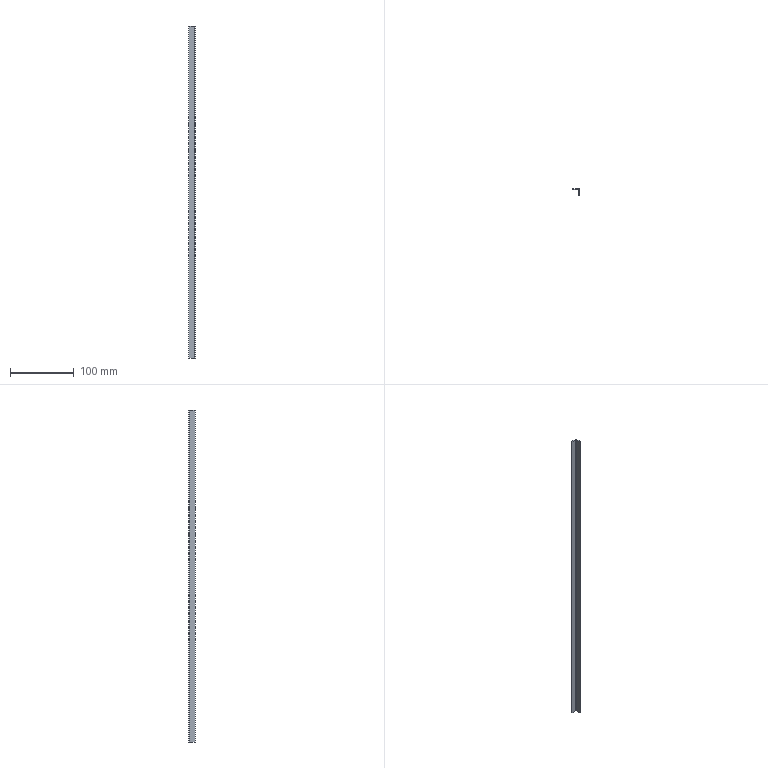Part | STEP file | 0001 | 1 solid | 14 faces | box 10 x 10 x 520 mm | volume 9724 mm3 | plane 12 | cylinder 2 | commonest cylinder face diameters 0.4 x1 2.4 x1
STEP:
#1=CARTESIAN_POINT('',(0.,0.,0.));
#2=DIRECTION('',(0.,0.,1.));
#3=DIRECTION('',(1.,0.,0.));
#4=AXIS2_PLACEMENT_3D('',#1,#2,#3);
#5=CARTESIAN_POINT('',(-1.2,0.,260.));
#6=VERTEX_POINT('',#5);
#7=CARTESIAN_POINT('',(-1.2,0.,-260.));
#8=VERTEX_POINT('',#7);
#9=CARTESIAN_POINT('',(-1.2,0.,260.));
#10=DIRECTION('',(0.,0.,-1.));
#11=VECTOR('',#10,1.);
#12=LINE('',#9,#11);
#13=CARTESIAN_POINT('',(0.,0.,-260.));
#14=DIRECTION('',(0.,1.,0.));
#15=DIRECTION('',(-1.,0.,0.));
#16=AXIS2_PLACEMENT_3D('',#13,#14,#15);
#17=PLANE('',#16);
#18=CARTESIAN_POINT('',(1.2,520.));
#19=DIRECTION('',(0.,-1.));
#20=VECTOR('',#19,1.);
#21=LINE('',#18,#20);
#22=(GEOMETRIC_REPRESENTATION_CONTEXT(2)PARAMETRIC_REPRESENTATION_CONTEXT()REPRESENTATION_CONTEXT('',''));
#23=DEFINITIONAL_REPRESENTATION('',(#21),#22);
#24=PCURVE('',#17,#23);
#25=CARTESIAN_POINT('',(-1.2,-1.2,937.872));
#26=DIRECTION('',(0.,0.,-1.));
#27=DIRECTION('',(0.,1.,0.));
#28=AXIS2_PLACEMENT_3D('',#25,#26,#27);
#29=CYLINDRICAL_SURFACE('',#28,1.2);
#30=CARTESIAN_POINT('',(0.,677.872));
#31=DIRECTION('',(0.,1.));
#32=VECTOR('',#31,1.);
#33=LINE('',#30,#32);
#34=(GEOMETRIC_REPRESENTATION_CONTEXT(2)PARAMETRIC_REPRESENTATION_CONTEXT()REPRESENTATION_CONTEXT('',''));
#35=DEFINITIONAL_REPRESENTATION('',(#33),#34);
#36=PCURVE('',#29,#35);
#37=SURFACE_CURVE('',#12,(#24,#36),.PCURVE_S1.);
#38=EDGE_CURVE('',#6,#8,#37,.T.);
#39=ORIENTED_EDGE('',*,*,#38,.F.);
#40=CARTESIAN_POINT('',(-10.,0.,260.));
#41=VERTEX_POINT('',#40);
#42=CARTESIAN_POINT('',(-1.2,0.,260.));
#43=DIRECTION('',(-1.,0.,0.));
#44=VECTOR('',#43,1.);
#45=LINE('',#42,#44);
#46=CARTESIAN_POINT('',(1.2,520.));
#47=DIRECTION('',(1.,0.));
#48=VECTOR('',#47,1.);
#49=LINE('',#46,#48);
#50=(GEOMETRIC_REPRESENTATION_CONTEXT(2)PARAMETRIC_REPRESENTATION_CONTEXT()REPRESENTATION_CONTEXT('',''));
#51=DEFINITIONAL_REPRESENTATION('',(#49),#50);
#52=PCURVE('',#17,#51);
#53=CARTESIAN_POINT('',(-5.25,-0.5,260.));
#54=DIRECTION('',(0.,0.,-1.));
#55=DIRECTION('',(-1.,0.,0.));
#56=AXIS2_PLACEMENT_3D('',#53,#54,#55);
#57=PLANE('',#56);
#58=CARTESIAN_POINT('',(-4.05,0.5));
#59=DIRECTION('',(1.,0.));
#60=VECTOR('',#59,1.);
#61=LINE('',#58,#60);
#62=(GEOMETRIC_REPRESENTATION_CONTEXT(2)PARAMETRIC_REPRESENTATION_CONTEXT()REPRESENTATION_CONTEXT('',''));
#63=DEFINITIONAL_REPRESENTATION('',(#61),#62);
#64=PCURVE('',#57,#63);
#65=SURFACE_CURVE('',#45,(#52,#64),.PCURVE_S1.);
#66=EDGE_CURVE('',#6,#41,#65,.T.);
#67=ORIENTED_EDGE('',*,*,#66,.T.);
#68=CARTESIAN_POINT('',(-10.,0.,-260.));
#69=VERTEX_POINT('',#68);
#70=CARTESIAN_POINT('',(-10.,0.,-260.));
#71=DIRECTION('',(0.,0.,1.));
#72=VECTOR('',#71,1.);
#73=LINE('',#70,#72);
#74=CARTESIAN_POINT('',(10.,0.));
#75=DIRECTION('',(0.,1.));
#76=VECTOR('',#75,1.);
#77=LINE('',#74,#76);
#78=(GEOMETRIC_REPRESENTATION_CONTEXT(2)PARAMETRIC_REPRESENTATION_CONTEXT()REPRESENTATION_CONTEXT('',''));
#79=DEFINITIONAL_REPRESENTATION('',(#77),#78);
#80=PCURVE('',#17,#79);
#81=CARTESIAN_POINT('',(-10.,-0.5,0.));
#82=DIRECTION('',(-1.,0.,0.));
#83=DIRECTION('',(0.,0.,1.));
#84=AXIS2_PLACEMENT_3D('',#81,#82,#83);
#85=PLANE('',#84);
#86=CARTESIAN_POINT('',(-260.,0.5));
#87=DIRECTION('',(1.,0.));
#88=VECTOR('',#87,1.);
#89=LINE('',#86,#88);
#90=(GEOMETRIC_REPRESENTATION_CONTEXT(2)PARAMETRIC_REPRESENTATION_CONTEXT()REPRESENTATION_CONTEXT('',''));
#91=DEFINITIONAL_REPRESENTATION('',(#89),#90);
#92=PCURVE('',#85,#91);
#93=SURFACE_CURVE('',#73,(#80,#92),.PCURVE_S1.);
#94=EDGE_CURVE('',#69,#41,#93,.T.);
#95=ORIENTED_EDGE('',*,*,#94,.F.);
#96=CARTESIAN_POINT('',(-1.2,0.,-260.));
#97=DIRECTION('',(-1.,0.,0.));
#98=VECTOR('',#97,1.);
#99=LINE('',#96,#98);
#100=CARTESIAN_POINT('',(1.2,0.));
#101=DIRECTION('',(1.,0.));
#102=VECTOR('',#101,1.);
#103=LINE('',#100,#102);
#104=(GEOMETRIC_REPRESENTATION_CONTEXT(2)PARAMETRIC_REPRESENTATION_CONTEXT()REPRESENTATION_CONTEXT('',''));
#105=DEFINITIONAL_REPRESENTATION('',(#103),#104);
#106=PCURVE('',#17,#105);
#107=CARTESIAN_POINT('',(-5.25,-0.5,-260.));
#108=DIRECTION('',(0.,0.,-1.));
#109=DIRECTION('',(-1.,0.,0.));
#110=AXIS2_PLACEMENT_3D('',#107,#108,#109);
#111=PLANE('',#110);
#112=CARTESIAN_POINT('',(-4.05,0.5));
#113=DIRECTION('',(1.,0.));
#114=VECTOR('',#113,1.);
#115=LINE('',#112,#114);
#116=(GEOMETRIC_REPRESENTATION_CONTEXT(2)PARAMETRIC_REPRESENTATION_CONTEXT()REPRESENTATION_CONTEXT('',''));
#117=DEFINITIONAL_REPRESENTATION('',(#115),#116);
#118=PCURVE('',#111,#117);
#119=SURFACE_CURVE('',#99,(#106,#118),.PCURVE_S1.);
#120=EDGE_CURVE('',#8,#69,#119,.T.);
#121=ORIENTED_EDGE('',*,*,#120,.F.);
#122=EDGE_LOOP('',(#39,#67,#95,#121));
#123=FACE_BOUND('',#122,.F.);
#124=ADVANCED_FACE('',(#123),#17,.T.);
#125=CARTESIAN_POINT('',(0.,-1.2,-260.));
#126=VERTEX_POINT('',#125);
#127=CARTESIAN_POINT('',(-1.2,-1.2,-260.));
#128=DIRECTION('',(0.,0.,-1.));
#129=DIRECTION('',(0.,1.,0.));
#130=AXIS2_PLACEMENT_3D('',#127,#128,#129);
#131=CIRCLE('',#130,1.2);
#132=CARTESIAN_POINT('',(0.,1197.872));
#133=DIRECTION('',(1.,0.));
#134=VECTOR('',#133,1.);
#135=LINE('',#132,#134);
#136=(GEOMETRIC_REPRESENTATION_CONTEXT(2)PARAMETRIC_REPRESENTATION_CONTEXT()REPRESENTATION_CONTEXT('',''));
#137=DEFINITIONAL_REPRESENTATION('',(#135),#136);
#138=PCURVE('',#29,#137);
#139=CARTESIAN_POINT('',(-0.705,-0.705,-260.));
#140=DIRECTION('',(0.,0.,1.));
#141=DIRECTION('',(1.,0.,0.));
#142=AXIS2_PLACEMENT_3D('',#139,#140,#141);
#143=PLANE('',#142);
#144=CARTESIAN_POINT('',(-0.495,0.705));
#145=CARTESIAN_POINT('',(1.583,0.705));
#146=CARTESIAN_POINT('',(0.5443,-1.095));
#147=CARTESIAN_POINT('',(-0.495,-2.895));
#148=CARTESIAN_POINT('',(-1.534,-1.095));
#149=CARTESIAN_POINT('',(-2.573,0.705));
#150=CARTESIAN_POINT('',(-0.495,0.705));
#151=(BOUNDED_CURVE()B_SPLINE_CURVE(2,(#144,#145,#146,#147,#148,#149,#150),.UNSPECIFIED.,.T.,.F.)B_SPLINE_CURVE_WITH_KNOTS((1,2,2,2,2,1),(-2.094,0.,2.094,4.189,6.283,8.378),.UNSPECIFIED.)CURVE()GEOMETRIC_REPRESENTATION_ITEM()RATIONAL_B_SPLINE_CURVE((1.,0.5,1.,0.5,1.,0.5,1.))REPRESENTATION_ITEM(''));
#152=(GEOMETRIC_REPRESENTATION_CONTEXT(2)PARAMETRIC_REPRESENTATION_CONTEXT()REPRESENTATION_CONTEXT('',''));
#153=DEFINITIONAL_REPRESENTATION('',(#151),#152);
#154=PCURVE('',#143,#153);
#155=SURFACE_CURVE('',#131,(#138,#154),.PCURVE_S1.);
#156=EDGE_CURVE('',#8,#126,#155,.T.);
#157=ORIENTED_EDGE('',*,*,#156,.F.);
#158=ORIENTED_EDGE('',*,*,#38,.F.);
#159=CARTESIAN_POINT('',(0.,-1.2,260.));
#160=VERTEX_POINT('',#159);
#161=CARTESIAN_POINT('',(-1.2,-1.2,260.));
#162=DIRECTION('',(0.,0.,1.));
#163=DIRECTION('',(1.,0.,0.));
#164=AXIS2_PLACEMENT_3D('',#161,#162,#163);
#165=CIRCLE('',#164,1.2);
#166=CARTESIAN_POINT('',(1.571,677.872));
#167=DIRECTION('',(-1.,0.));
#168=VECTOR('',#167,1.);
#169=LINE('',#166,#168);
#170=(GEOMETRIC_REPRESENTATION_CONTEXT(2)PARAMETRIC_REPRESENTATION_CONTEXT()REPRESENTATION_CONTEXT('',''));
#171=DEFINITIONAL_REPRESENTATION('',(#169),#170);
#172=PCURVE('',#29,#171);
#173=CARTESIAN_POINT('',(-0.705,-0.705,260.));
#174=DIRECTION('',(0.,0.,-1.));
#175=DIRECTION('',(0.,1.,0.));
#176=AXIS2_PLACEMENT_3D('',#173,#174,#175);
#177=PLANE('',#176);
#178=CARTESIAN_POINT('',(-0.495,0.705));
#179=CARTESIAN_POINT('',(1.583,0.705));
#180=CARTESIAN_POINT('',(0.5443,-1.095));
#181=CARTESIAN_POINT('',(-0.495,-2.895));
#182=CARTESIAN_POINT('',(-1.534,-1.095));
#183=CARTESIAN_POINT('',(-2.573,0.705));
#184=CARTESIAN_POINT('',(-0.495,0.705));
#185=(BOUNDED_CURVE()B_SPLINE_CURVE(2,(#178,#179,#180,#181,#182,#183,#184),.UNSPECIFIED.,.T.,.F.)B_SPLINE_CURVE_WITH_KNOTS((1,2,2,2,2,1),(-2.094,0.,2.094,4.189,6.283,8.378),.UNSPECIFIED.)CURVE()GEOMETRIC_REPRESENTATION_ITEM()RATIONAL_B_SPLINE_CURVE((1.,0.5,1.,0.5,1.,0.5,1.))REPRESENTATION_ITEM(''));
#186=(GEOMETRIC_REPRESENTATION_CONTEXT(2)PARAMETRIC_REPRESENTATION_CONTEXT()REPRESENTATION_CONTEXT('',''));
#187=DEFINITIONAL_REPRESENTATION('',(#185),#186);
#188=PCURVE('',#177,#187);
#189=SURFACE_CURVE('',#165,(#172,#188),.PCURVE_S1.);
#190=EDGE_CURVE('',#160,#6,#189,.T.);
#191=ORIENTED_EDGE('',*,*,#190,.F.);
#192=CARTESIAN_POINT('',(0.,-1.2,260.));
#193=DIRECTION('',(0.,0.,-1.));
#194=VECTOR('',#193,1.);
#195=LINE('',#192,#194);
#196=CARTESIAN_POINT('',(1.571,677.872));
#197=DIRECTION('',(0.,1.));
#198=VECTOR('',#197,1.);
#199=LINE('',#196,#198);
#200=(GEOMETRIC_REPRESENTATION_CONTEXT(2)PARAMETRIC_REPRESENTATION_CONTEXT()REPRESENTATION_CONTEXT('',''));
#201=DEFINITIONAL_REPRESENTATION('',(#199),#200);
#202=PCURVE('',#29,#201);
#203=CARTESIAN_POINT('',(0.,-10.,-260.));
#204=DIRECTION('',(1.,0.,0.));
#205=DIRECTION('',(0.,1.,0.));
#206=AXIS2_PLACEMENT_3D('',#203,#204,#205);
#207=PLANE('',#206);
#208=CARTESIAN_POINT('',(8.8,520.));
#209=DIRECTION('',(0.,-1.));
#210=VECTOR('',#209,1.);
#211=LINE('',#208,#210);
#212=(GEOMETRIC_REPRESENTATION_CONTEXT(2)PARAMETRIC_REPRESENTATION_CONTEXT()REPRESENTATION_CONTEXT('',''));
#213=DEFINITIONAL_REPRESENTATION('',(#211),#212);
#214=PCURVE('',#207,#213);
#215=SURFACE_CURVE('',#195,(#202,#214),.PCURVE_S1.);
#216=EDGE_CURVE('',#160,#126,#215,.T.);
#217=ORIENTED_EDGE('',*,*,#216,.T.);
#218=EDGE_LOOP('',(#157,#158,#191,#217));
#219=FACE_BOUND('',#218,.T.);
#220=ADVANCED_FACE('',(#219),#29,.T.);
#221=ORIENTED_EDGE('',*,*,#216,.T.);
#222=CARTESIAN_POINT('',(0.,-10.,-260.));
#223=VERTEX_POINT('',#222);
#224=CARTESIAN_POINT('',(0.,-10.,-260.));
#225=DIRECTION('',(0.,1.,0.));
#226=VECTOR('',#225,1.);
#227=LINE('',#224,#226);
#228=CARTESIAN_POINT('',(0.,0.));
#229=DIRECTION('',(1.,0.));
#230=VECTOR('',#229,1.);
#231=LINE('',#228,#230);
#232=(GEOMETRIC_REPRESENTATION_CONTEXT(2)PARAMETRIC_REPRESENTATION_CONTEXT()REPRESENTATION_CONTEXT('',''));
#233=DEFINITIONAL_REPRESENTATION('',(#231),#232);
#234=PCURVE('',#207,#233);
#235=CARTESIAN_POINT('',(-0.5,-5.25,-260.));
#236=DIRECTION('',(0.,0.,-1.));
#237=DIRECTION('',(0.,1.,0.));
#238=AXIS2_PLACEMENT_3D('',#235,#236,#237);
#239=PLANE('',#238);
#240=CARTESIAN_POINT('',(-4.75,0.5));
#241=DIRECTION('',(1.,0.));
#242=VECTOR('',#241,1.);
#243=LINE('',#240,#242);
#244=(GEOMETRIC_REPRESENTATION_CONTEXT(2)PARAMETRIC_REPRESENTATION_CONTEXT()REPRESENTATION_CONTEXT('',''));
#245=DEFINITIONAL_REPRESENTATION('',(#243),#244);
#246=PCURVE('',#239,#245);
#247=SURFACE_CURVE('',#227,(#234,#246),.PCURVE_S1.);
#248=EDGE_CURVE('',#223,#126,#247,.T.);
#249=ORIENTED_EDGE('',*,*,#248,.F.);
#250=CARTESIAN_POINT('',(0.,-10.,260.));
#251=VERTEX_POINT('',#250);
#252=CARTESIAN_POINT('',(0.,-10.,-260.));
#253=DIRECTION('',(0.,0.,1.));
#254=VECTOR('',#253,1.);
#255=LINE('',#252,#254);
#256=CARTESIAN_POINT('',(0.,0.));
#257=DIRECTION('',(0.,1.));
#258=VECTOR('',#257,1.);
#259=LINE('',#256,#258);
#260=(GEOMETRIC_REPRESENTATION_CONTEXT(2)PARAMETRIC_REPRESENTATION_CONTEXT()REPRESENTATION_CONTEXT('',''));
#261=DEFINITIONAL_REPRESENTATION('',(#259),#260);
#262=PCURVE('',#207,#261);
#263=CARTESIAN_POINT('',(-0.5,-10.,0.));
#264=DIRECTION('',(0.,1.,0.));
#265=DIRECTION('',(0.,0.,1.));
#266=AXIS2_PLACEMENT_3D('',#263,#264,#265);
#267=PLANE('',#266);
#268=CARTESIAN_POINT('',(-260.,0.5));
#269=DIRECTION('',(1.,0.));
#270=VECTOR('',#269,1.);
#271=LINE('',#268,#270);
#272=(GEOMETRIC_REPRESENTATION_CONTEXT(2)PARAMETRIC_REPRESENTATION_CONTEXT()REPRESENTATION_CONTEXT('',''));
#273=DEFINITIONAL_REPRESENTATION('',(#271),#272);
#274=PCURVE('',#267,#273);
#275=SURFACE_CURVE('',#255,(#262,#274),.PCURVE_S1.);
#276=EDGE_CURVE('',#223,#251,#275,.T.);
#277=ORIENTED_EDGE('',*,*,#276,.T.);
#278=CARTESIAN_POINT('',(0.,-10.,260.));
#279=DIRECTION('',(0.,1.,0.));
#280=VECTOR('',#279,1.);
#281=LINE('',#278,#280);
#282=CARTESIAN_POINT('',(0.,520.));
#283=DIRECTION('',(1.,0.));
#284=VECTOR('',#283,1.);
#285=LINE('',#282,#284);
#286=(GEOMETRIC_REPRESENTATION_CONTEXT(2)PARAMETRIC_REPRESENTATION_CONTEXT()REPRESENTATION_CONTEXT('',''));
#287=DEFINITIONAL_REPRESENTATION('',(#285),#286);
#288=PCURVE('',#207,#287);
#289=CARTESIAN_POINT('',(-0.5,-5.25,260.));
#290=DIRECTION('',(0.,0.,-1.));
#291=DIRECTION('',(0.,1.,0.));
#292=AXIS2_PLACEMENT_3D('',#289,#290,#291);
#293=PLANE('',#292);
#294=CARTESIAN_POINT('',(-4.75,0.5));
#295=DIRECTION('',(1.,0.));
#296=VECTOR('',#295,1.);
#297=LINE('',#294,#296);
#298=(GEOMETRIC_REPRESENTATION_CONTEXT(2)PARAMETRIC_REPRESENTATION_CONTEXT()REPRESENTATION_CONTEXT('',''));
#299=DEFINITIONAL_REPRESENTATION('',(#297),#298);
#300=PCURVE('',#293,#299);
#301=SURFACE_CURVE('',#281,(#288,#300),.PCURVE_S1.);
#302=EDGE_CURVE('',#251,#160,#301,.T.);
#303=ORIENTED_EDGE('',*,*,#302,.T.);
#304=EDGE_LOOP('',(#221,#249,#277,#303));
#305=FACE_BOUND('',#304,.F.);
#306=ADVANCED_FACE('',(#305),#207,.T.);
#307=CARTESIAN_POINT('',(-1.,-1.2,-260.));
#308=VERTEX_POINT('',#307);
#309=CARTESIAN_POINT('',(0.,-1.2,-260.));
#310=DIRECTION('',(-1.,0.,0.));
#311=VECTOR('',#310,1.);
#312=LINE('',#309,#311);
#313=CARTESIAN_POINT('',(4.05,0.5));
#314=DIRECTION('',(0.,-1.));
#315=VECTOR('',#314,1.);
#316=LINE('',#313,#315);
#317=(GEOMETRIC_REPRESENTATION_CONTEXT(2)PARAMETRIC_REPRESENTATION_CONTEXT()REPRESENTATION_CONTEXT('',''));
#318=DEFINITIONAL_REPRESENTATION('',(#316),#317);
#319=PCURVE('',#239,#318);
#320=CARTESIAN_POINT('',(0.705,-0.495));
#321=DIRECTION('',(-1.,0.));
#322=VECTOR('',#321,1.);
#323=LINE('',#320,#322);
#324=(GEOMETRIC_REPRESENTATION_CONTEXT(2)PARAMETRIC_REPRESENTATION_CONTEXT()REPRESENTATION_CONTEXT('',''));
#325=DEFINITIONAL_REPRESENTATION('',(#323),#324);
#326=PCURVE('',#143,#325);
#327=SURFACE_CURVE('',#312,(#319,#326),.PCURVE_S1.);
#328=EDGE_CURVE('',#126,#308,#327,.T.);
#329=ORIENTED_EDGE('',*,*,#328,.T.);
#330=CARTESIAN_POINT('',(-1.,-10.,-260.));
#331=VERTEX_POINT('',#330);
#332=CARTESIAN_POINT('',(-1.,-10.,-260.));
#333=DIRECTION('',(0.,1.,0.));
#334=VECTOR('',#333,1.);
#335=LINE('',#332,#334);
#336=CARTESIAN_POINT('',(-4.75,-0.5));
#337=DIRECTION('',(1.,0.));
#338=VECTOR('',#337,1.);
#339=LINE('',#336,#338);
#340=(GEOMETRIC_REPRESENTATION_CONTEXT(2)PARAMETRIC_REPRESENTATION_CONTEXT()REPRESENTATION_CONTEXT('',''));
#341=DEFINITIONAL_REPRESENTATION('',(#339),#340);
#342=PCURVE('',#239,#341);
#343=CARTESIAN_POINT('',(-1.,-10.,-260.));
#344=DIRECTION('',(1.,0.,0.));
#345=DIRECTION('',(0.,1.,0.));
#346=AXIS2_PLACEMENT_3D('',#343,#344,#345);
#347=PLANE('',#346);
#348=CARTESIAN_POINT('',(0.,0.));
#349=DIRECTION('',(1.,0.));
#350=VECTOR('',#349,1.);
#351=LINE('',#348,#350);
#352=(GEOMETRIC_REPRESENTATION_CONTEXT(2)PARAMETRIC_REPRESENTATION_CONTEXT()REPRESENTATION_CONTEXT('',''));
#353=DEFINITIONAL_REPRESENTATION('',(#351),#352);
#354=PCURVE('',#347,#353);
#355=SURFACE_CURVE('',#335,(#342,#354),.PCURVE_S1.);
#356=EDGE_CURVE('',#331,#308,#355,.T.);
#357=ORIENTED_EDGE('',*,*,#356,.F.);
#358=CARTESIAN_POINT('',(0.,-10.,-260.));
#359=DIRECTION('',(-1.,0.,0.));
#360=VECTOR('',#359,1.);
#361=LINE('',#358,#360);
#362=CARTESIAN_POINT('',(-4.75,0.5));
#363=DIRECTION('',(0.,-1.));
#364=VECTOR('',#363,1.);
#365=LINE('',#362,#364);
#366=(GEOMETRIC_REPRESENTATION_CONTEXT(2)PARAMETRIC_REPRESENTATION_CONTEXT()REPRESENTATION_CONTEXT('',''));
#367=DEFINITIONAL_REPRESENTATION('',(#365),#366);
#368=PCURVE('',#239,#367);
#369=CARTESIAN_POINT('',(-260.,0.5));
#370=DIRECTION('',(0.,-1.));
#371=VECTOR('',#370,1.);
#372=LINE('',#369,#371);
#373=(GEOMETRIC_REPRESENTATION_CONTEXT(2)PARAMETRIC_REPRESENTATION_CONTEXT()REPRESENTATION_CONTEXT('',''));
#374=DEFINITIONAL_REPRESENTATION('',(#372),#373);
#375=PCURVE('',#267,#374);
#376=SURFACE_CURVE('',#361,(#368,#375),.PCURVE_S1.);
#377=EDGE_CURVE('',#223,#331,#376,.T.);
#378=ORIENTED_EDGE('',*,*,#377,.F.);
#379=ORIENTED_EDGE('',*,*,#248,.T.);
#380=EDGE_LOOP('',(#329,#357,#378,#379));
#381=FACE_BOUND('',#380,.F.);
#382=ADVANCED_FACE('',(#381),#239,.T.);
#383=ORIENTED_EDGE('',*,*,#156,.F.);
#384=CARTESIAN_POINT('',(-1.2,-1.,-260.));
#385=VERTEX_POINT('',#384);
#386=CARTESIAN_POINT('',(-1.2,0.,-260.));
#387=DIRECTION('',(0.,-1.,0.));
#388=VECTOR('',#387,1.);
#389=LINE('',#386,#388);
#390=CARTESIAN_POINT('',(-0.495,0.705));
#391=DIRECTION('',(0.,-1.));
#392=VECTOR('',#391,1.);
#393=LINE('',#390,#392);
#394=(GEOMETRIC_REPRESENTATION_CONTEXT(2)PARAMETRIC_REPRESENTATION_CONTEXT()REPRESENTATION_CONTEXT('',''));
#395=DEFINITIONAL_REPRESENTATION('',(#393),#394);
#396=PCURVE('',#143,#395);
#397=CARTESIAN_POINT('',(-4.05,0.5));
#398=DIRECTION('',(0.,-1.));
#399=VECTOR('',#398,1.);
#400=LINE('',#397,#399);
#401=(GEOMETRIC_REPRESENTATION_CONTEXT(2)PARAMETRIC_REPRESENTATION_CONTEXT()REPRESENTATION_CONTEXT('',''));
#402=DEFINITIONAL_REPRESENTATION('',(#400),#401);
#403=PCURVE('',#111,#402);
#404=SURFACE_CURVE('',#389,(#396,#403),.PCURVE_S1.);
#405=EDGE_CURVE('',#8,#385,#404,.T.);
#406=ORIENTED_EDGE('',*,*,#405,.T.);
#407=CARTESIAN_POINT('',(-1.2,-1.2,-260.));
#408=DIRECTION('',(0.,0.,-1.));
#409=DIRECTION('',(0.,1.,0.));
#410=AXIS2_PLACEMENT_3D('',#407,#408,#409);
#411=CIRCLE('',#410,0.2);
#412=CARTESIAN_POINT('',(-0.495,-0.295));
#413=CARTESIAN_POINT('',(-0.1486,-0.295));
#414=CARTESIAN_POINT('',(-0.3218,-0.595));
#415=CARTESIAN_POINT('',(-0.495,-0.895));
#416=CARTESIAN_POINT('',(-0.6682,-0.595));
#417=CARTESIAN_POINT('',(-0.8414,-0.295));
#418=CARTESIAN_POINT('',(-0.495,-0.295));
#419=(BOUNDED_CURVE()B_SPLINE_CURVE(2,(#412,#413,#414,#415,#416,#417,#418),.UNSPECIFIED.,.T.,.F.)B_SPLINE_CURVE_WITH_KNOTS((1,2,2,2,2,1),(-2.094,0.,2.094,4.189,6.283,8.378),.UNSPECIFIED.)CURVE()GEOMETRIC_REPRESENTATION_ITEM()RATIONAL_B_SPLINE_CURVE((1.,0.5,1.,0.5,1.,0.5,1.))REPRESENTATION_ITEM(''));
#420=(GEOMETRIC_REPRESENTATION_CONTEXT(2)PARAMETRIC_REPRESENTATION_CONTEXT()REPRESENTATION_CONTEXT('',''));
#421=DEFINITIONAL_REPRESENTATION('',(#419),#420);
#422=PCURVE('',#143,#421);
#423=CARTESIAN_POINT('',(-1.2,-1.2,937.872));
#424=DIRECTION('',(0.,0.,-1.));
#425=DIRECTION('',(0.,1.,0.));
#426=AXIS2_PLACEMENT_3D('',#423,#424,#425);
#427=CYLINDRICAL_SURFACE('',#426,0.2);
#428=CARTESIAN_POINT('',(0.,1197.872));
#429=DIRECTION('',(1.,0.));
#430=VECTOR('',#429,1.);
#431=LINE('',#428,#430);
#432=(GEOMETRIC_REPRESENTATION_CONTEXT(2)PARAMETRIC_REPRESENTATION_CONTEXT()REPRESENTATION_CONTEXT('',''));
#433=DEFINITIONAL_REPRESENTATION('',(#431),#432);
#434=PCURVE('',#427,#433);
#435=SURFACE_CURVE('',#411,(#422,#434),.PCURVE_S1.);
#436=EDGE_CURVE('',#385,#308,#435,.T.);
#437=ORIENTED_EDGE('',*,*,#436,.T.);
#438=ORIENTED_EDGE('',*,*,#328,.F.);
#439=EDGE_LOOP('',(#383,#406,#437,#438));
#440=FACE_BOUND('',#439,.F.);
#441=ADVANCED_FACE('',(#440),#143,.F.);
#442=ORIENTED_EDGE('',*,*,#405,.F.);
#443=ORIENTED_EDGE('',*,*,#120,.T.);
#444=CARTESIAN_POINT('',(-10.,-1.,-260.));
#445=VERTEX_POINT('',#444);
#446=CARTESIAN_POINT('',(-10.,0.,-260.));
#447=DIRECTION('',(0.,-1.,0.));
#448=VECTOR('',#447,1.);
#449=LINE('',#446,#448);
#450=CARTESIAN_POINT('',(4.75,0.5));
#451=DIRECTION('',(0.,-1.));
#452=VECTOR('',#451,1.);
#453=LINE('',#450,#452);
#454=(GEOMETRIC_REPRESENTATION_CONTEXT(2)PARAMETRIC_REPRESENTATION_CONTEXT()REPRESENTATION_CONTEXT('',''));
#455=DEFINITIONAL_REPRESENTATION('',(#453),#454);
#456=PCURVE('',#111,#455);
#457=CARTESIAN_POINT('',(-260.,0.5));
#458=DIRECTION('',(0.,-1.));
#459=VECTOR('',#458,1.);
#460=LINE('',#457,#459);
#461=(GEOMETRIC_REPRESENTATION_CONTEXT(2)PARAMETRIC_REPRESENTATION_CONTEXT()REPRESENTATION_CONTEXT('',''));
#462=DEFINITIONAL_REPRESENTATION('',(#460),#461);
#463=PCURVE('',#85,#462);
#464=SURFACE_CURVE('',#449,(#456,#463),.PCURVE_S1.);
#465=EDGE_CURVE('',#69,#445,#464,.T.);
#466=ORIENTED_EDGE('',*,*,#465,.T.);
#467=CARTESIAN_POINT('',(-1.2,-1.,-260.));
#468=DIRECTION('',(-1.,0.,0.));
#469=VECTOR('',#468,1.);
#470=LINE('',#467,#469);
#471=CARTESIAN_POINT('',(-4.05,-0.5));
#472=DIRECTION('',(1.,0.));
#473=VECTOR('',#472,1.);
#474=LINE('',#471,#473);
#475=(GEOMETRIC_REPRESENTATION_CONTEXT(2)PARAMETRIC_REPRESENTATION_CONTEXT()REPRESENTATION_CONTEXT('',''));
#476=DEFINITIONAL_REPRESENTATION('',(#474),#475);
#477=PCURVE('',#111,#476);
#478=CARTESIAN_POINT('',(0.,-1.,-260.));
#479=DIRECTION('',(0.,1.,0.));
#480=DIRECTION('',(-1.,0.,0.));
#481=AXIS2_PLACEMENT_3D('',#478,#479,#480);
#482=PLANE('',#481);
#483=CARTESIAN_POINT('',(1.2,0.));
#484=DIRECTION('',(1.,0.));
#485=VECTOR('',#484,1.);
#486=LINE('',#483,#485);
#487=(GEOMETRIC_REPRESENTATION_CONTEXT(2)PARAMETRIC_REPRESENTATION_CONTEXT()REPRESENTATION_CONTEXT('',''));
#488=DEFINITIONAL_REPRESENTATION('',(#486),#487);
#489=PCURVE('',#482,#488);
#490=SURFACE_CURVE('',#470,(#477,#489),.PCURVE_S1.);
#491=EDGE_CURVE('',#385,#445,#490,.T.);
#492=ORIENTED_EDGE('',*,*,#491,.F.);
#493=EDGE_LOOP('',(#442,#443,#466,#492));
#494=FACE_BOUND('',#493,.F.);
#495=ADVANCED_FACE('',(#494),#111,.T.);
#496=ORIENTED_EDGE('',*,*,#94,.T.);
#497=CARTESIAN_POINT('',(-10.,-1.,260.));
#498=VERTEX_POINT('',#497);
#499=CARTESIAN_POINT('',(-10.,0.,260.));
#500=DIRECTION('',(0.,-1.,0.));
#501=VECTOR('',#500,1.);
#502=LINE('',#499,#501);
#503=CARTESIAN_POINT('',(260.,0.5));
#504=DIRECTION('',(0.,-1.));
#505=VECTOR('',#504,1.);
#506=LINE('',#503,#505);
#507=(GEOMETRIC_REPRESENTATION_CONTEXT(2)PARAMETRIC_REPRESENTATION_CONTEXT()REPRESENTATION_CONTEXT('',''));
#508=DEFINITIONAL_REPRESENTATION('',(#506),#507);
#509=PCURVE('',#85,#508);
#510=CARTESIAN_POINT('',(4.75,0.5));
#511=DIRECTION('',(0.,-1.));
#512=VECTOR('',#511,1.);
#513=LINE('',#510,#512);
#514=(GEOMETRIC_REPRESENTATION_CONTEXT(2)PARAMETRIC_REPRESENTATION_CONTEXT()REPRESENTATION_CONTEXT('',''));
#515=DEFINITIONAL_REPRESENTATION('',(#513),#514);
#516=PCURVE('',#57,#515);
#517=SURFACE_CURVE('',#502,(#509,#516),.PCURVE_S1.);
#518=EDGE_CURVE('',#41,#498,#517,.T.);
#519=ORIENTED_EDGE('',*,*,#518,.T.);
#520=CARTESIAN_POINT('',(-10.,-1.,-260.));
#521=DIRECTION('',(0.,0.,1.));
#522=VECTOR('',#521,1.);
#523=LINE('',#520,#522);
#524=CARTESIAN_POINT('',(-260.,-0.5));
#525=DIRECTION('',(1.,0.));
#526=VECTOR('',#525,1.);
#527=LINE('',#524,#526);
#528=(GEOMETRIC_REPRESENTATION_CONTEXT(2)PARAMETRIC_REPRESENTATION_CONTEXT()REPRESENTATION_CONTEXT('',''));
#529=DEFINITIONAL_REPRESENTATION('',(#527),#528);
#530=PCURVE('',#85,#529);
#531=CARTESIAN_POINT('',(10.,0.));
#532=DIRECTION('',(0.,1.));
#533=VECTOR('',#532,1.);
#534=LINE('',#531,#533);
#535=(GEOMETRIC_REPRESENTATION_CONTEXT(2)PARAMETRIC_REPRESENTATION_CONTEXT()REPRESENTATION_CONTEXT('',''));
#536=DEFINITIONAL_REPRESENTATION('',(#534),#535);
#537=PCURVE('',#482,#536);
#538=SURFACE_CURVE('',#523,(#530,#537),.PCURVE_S1.);
#539=EDGE_CURVE('',#445,#498,#538,.T.);
#540=ORIENTED_EDGE('',*,*,#539,.F.);
#541=ORIENTED_EDGE('',*,*,#465,.F.);
#542=EDGE_LOOP('',(#496,#519,#540,#541));
#543=FACE_BOUND('',#542,.F.);
#544=ADVANCED_FACE('',(#543),#85,.T.);
#545=CARTESIAN_POINT('',(-1.2,-1.,260.));
#546=VERTEX_POINT('',#545);
#547=CARTESIAN_POINT('',(-1.2,0.,260.));
#548=DIRECTION('',(0.,-1.,0.));
#549=VECTOR('',#548,1.);
#550=LINE('',#547,#549);
#551=CARTESIAN_POINT('',(-4.05,0.5));
#552=DIRECTION('',(0.,-1.));
#553=VECTOR('',#552,1.);
#554=LINE('',#551,#553);
#555=(GEOMETRIC_REPRESENTATION_CONTEXT(2)PARAMETRIC_REPRESENTATION_CONTEXT()REPRESENTATION_CONTEXT('',''));
#556=DEFINITIONAL_REPRESENTATION('',(#554),#555);
#557=PCURVE('',#57,#556);
#558=CARTESIAN_POINT('',(0.705,-0.495));
#559=DIRECTION('',(-1.,0.));
#560=VECTOR('',#559,1.);
#561=LINE('',#558,#560);
#562=(GEOMETRIC_REPRESENTATION_CONTEXT(2)PARAMETRIC_REPRESENTATION_CONTEXT()REPRESENTATION_CONTEXT('',''));
#563=DEFINITIONAL_REPRESENTATION('',(#561),#562);
#564=PCURVE('',#177,#563);
#565=SURFACE_CURVE('',#550,(#557,#564),.PCURVE_S1.);
#566=EDGE_CURVE('',#6,#546,#565,.T.);
#567=ORIENTED_EDGE('',*,*,#566,.T.);
#568=CARTESIAN_POINT('',(-1.2,-1.,260.));
#569=DIRECTION('',(-1.,0.,0.));
#570=VECTOR('',#569,1.);
#571=LINE('',#568,#570);
#572=CARTESIAN_POINT('',(-4.05,-0.5));
#573=DIRECTION('',(1.,0.));
#574=VECTOR('',#573,1.);
#575=LINE('',#572,#574);
#576=(GEOMETRIC_REPRESENTATION_CONTEXT(2)PARAMETRIC_REPRESENTATION_CONTEXT()REPRESENTATION_CONTEXT('',''));
#577=DEFINITIONAL_REPRESENTATION('',(#575),#576);
#578=PCURVE('',#57,#577);
#579=CARTESIAN_POINT('',(1.2,520.));
#580=DIRECTION('',(1.,0.));
#581=VECTOR('',#580,1.);
#582=LINE('',#579,#581);
#583=(GEOMETRIC_REPRESENTATION_CONTEXT(2)PARAMETRIC_REPRESENTATION_CONTEXT()REPRESENTATION_CONTEXT('',''));
#584=DEFINITIONAL_REPRESENTATION('',(#582),#583);
#585=PCURVE('',#482,#584);
#586=SURFACE_CURVE('',#571,(#578,#585),.PCURVE_S1.);
#587=EDGE_CURVE('',#546,#498,#586,.T.);
#588=ORIENTED_EDGE('',*,*,#587,.T.);
#589=ORIENTED_EDGE('',*,*,#518,.F.);
#590=ORIENTED_EDGE('',*,*,#66,.F.);
#591=EDGE_LOOP('',(#567,#588,#589,#590));
#592=FACE_BOUND('',#591,.F.);
#593=ADVANCED_FACE('',(#592),#57,.F.);
#594=ORIENTED_EDGE('',*,*,#190,.F.);
#595=CARTESIAN_POINT('',(-1.,-1.2,260.));
#596=VERTEX_POINT('',#595);
#597=CARTESIAN_POINT('',(0.,-1.2,260.));
#598=DIRECTION('',(-1.,0.,0.));
#599=VECTOR('',#598,1.);
#600=LINE('',#597,#599);
#601=CARTESIAN_POINT('',(-0.495,0.705));
#602=DIRECTION('',(0.,-1.));
#603=VECTOR('',#602,1.);
#604=LINE('',#601,#603);
#605=(GEOMETRIC_REPRESENTATION_CONTEXT(2)PARAMETRIC_REPRESENTATION_CONTEXT()REPRESENTATION_CONTEXT('',''));
#606=DEFINITIONAL_REPRESENTATION('',(#604),#605);
#607=PCURVE('',#177,#606);
#608=CARTESIAN_POINT('',(4.05,0.5));
#609=DIRECTION('',(0.,-1.));
#610=VECTOR('',#609,1.);
#611=LINE('',#608,#610);
#612=(GEOMETRIC_REPRESENTATION_CONTEXT(2)PARAMETRIC_REPRESENTATION_CONTEXT()REPRESENTATION_CONTEXT('',''));
#613=DEFINITIONAL_REPRESENTATION('',(#611),#612);
#614=PCURVE('',#293,#613);
#615=SURFACE_CURVE('',#600,(#607,#614),.PCURVE_S1.);
#616=EDGE_CURVE('',#160,#596,#615,.T.);
#617=ORIENTED_EDGE('',*,*,#616,.T.);
#618=CARTESIAN_POINT('',(-1.2,-1.2,260.));
#619=DIRECTION('',(0.,0.,1.));
#620=DIRECTION('',(1.,0.,0.));
#621=AXIS2_PLACEMENT_3D('',#618,#619,#620);
#622=CIRCLE('',#621,0.2);
#623=CARTESIAN_POINT('',(-0.495,-0.295));
#624=CARTESIAN_POINT('',(-0.1486,-0.295));
#625=CARTESIAN_POINT('',(-0.3218,-0.595));
#626=CARTESIAN_POINT('',(-0.495,-0.895));
#627=CARTESIAN_POINT('',(-0.6682,-0.595));
#628=CARTESIAN_POINT('',(-0.8414,-0.295));
#629=CARTESIAN_POINT('',(-0.495,-0.295));
#630=(BOUNDED_CURVE()B_SPLINE_CURVE(2,(#623,#624,#625,#626,#627,#628,#629),.UNSPECIFIED.,.T.,.F.)B_SPLINE_CURVE_WITH_KNOTS((1,2,2,2,2,1),(-2.094,0.,2.094,4.189,6.283,8.378),.UNSPECIFIED.)CURVE()GEOMETRIC_REPRESENTATION_ITEM()RATIONAL_B_SPLINE_CURVE((1.,0.5,1.,0.5,1.,0.5,1.))REPRESENTATION_ITEM(''));
#631=(GEOMETRIC_REPRESENTATION_CONTEXT(2)PARAMETRIC_REPRESENTATION_CONTEXT()REPRESENTATION_CONTEXT('',''));
#632=DEFINITIONAL_REPRESENTATION('',(#630),#631);
#633=PCURVE('',#177,#632);
#634=CARTESIAN_POINT('',(1.571,677.872));
#635=DIRECTION('',(-1.,0.));
#636=VECTOR('',#635,1.);
#637=LINE('',#634,#636);
#638=(GEOMETRIC_REPRESENTATION_CONTEXT(2)PARAMETRIC_REPRESENTATION_CONTEXT()REPRESENTATION_CONTEXT('',''));
#639=DEFINITIONAL_REPRESENTATION('',(#637),#638);
#640=PCURVE('',#427,#639);
#641=SURFACE_CURVE('',#622,(#633,#640),.PCURVE_S1.);
#642=EDGE_CURVE('',#596,#546,#641,.T.);
#643=ORIENTED_EDGE('',*,*,#642,.T.);
#644=ORIENTED_EDGE('',*,*,#566,.F.);
#645=EDGE_LOOP('',(#594,#617,#643,#644));
#646=FACE_BOUND('',#645,.F.);
#647=ADVANCED_FACE('',(#646),#177,.F.);
#648=ORIENTED_EDGE('',*,*,#616,.F.);
#649=ORIENTED_EDGE('',*,*,#302,.F.);
#650=CARTESIAN_POINT('',(-1.,-10.,260.));
#651=VERTEX_POINT('',#650);
#652=CARTESIAN_POINT('',(0.,-10.,260.));
#653=DIRECTION('',(-1.,0.,0.));
#654=VECTOR('',#653,1.);
#655=LINE('',#652,#654);
#656=CARTESIAN_POINT('',(-4.75,0.5));
#657=DIRECTION('',(0.,-1.));
#658=VECTOR('',#657,1.);
#659=LINE('',#656,#658);
#660=(GEOMETRIC_REPRESENTATION_CONTEXT(2)PARAMETRIC_REPRESENTATION_CONTEXT()REPRESENTATION_CONTEXT('',''));
#661=DEFINITIONAL_REPRESENTATION('',(#659),#660);
#662=PCURVE('',#293,#661);
#663=CARTESIAN_POINT('',(260.,0.5));
#664=DIRECTION('',(0.,-1.));
#665=VECTOR('',#664,1.);
#666=LINE('',#663,#665);
#667=(GEOMETRIC_REPRESENTATION_CONTEXT(2)PARAMETRIC_REPRESENTATION_CONTEXT()REPRESENTATION_CONTEXT('',''));
#668=DEFINITIONAL_REPRESENTATION('',(#666),#667);
#669=PCURVE('',#267,#668);
#670=SURFACE_CURVE('',#655,(#662,#669),.PCURVE_S1.);
#671=EDGE_CURVE('',#251,#651,#670,.T.);
#672=ORIENTED_EDGE('',*,*,#671,.T.);
#673=CARTESIAN_POINT('',(-1.,-10.,260.));
#674=DIRECTION('',(0.,1.,0.));
#675=VECTOR('',#674,1.);
#676=LINE('',#673,#675);
#677=CARTESIAN_POINT('',(-4.75,-0.5));
#678=DIRECTION('',(1.,0.));
#679=VECTOR('',#678,1.);
#680=LINE('',#677,#679);
#681=(GEOMETRIC_REPRESENTATION_CONTEXT(2)PARAMETRIC_REPRESENTATION_CONTEXT()REPRESENTATION_CONTEXT('',''));
#682=DEFINITIONAL_REPRESENTATION('',(#680),#681);
#683=PCURVE('',#293,#682);
#684=CARTESIAN_POINT('',(0.,520.));
#685=DIRECTION('',(1.,0.));
#686=VECTOR('',#685,1.);
#687=LINE('',#684,#686);
#688=(GEOMETRIC_REPRESENTATION_CONTEXT(2)PARAMETRIC_REPRESENTATION_CONTEXT()REPRESENTATION_CONTEXT('',''));
#689=DEFINITIONAL_REPRESENTATION('',(#687),#688);
#690=PCURVE('',#347,#689);
#691=SURFACE_CURVE('',#676,(#683,#690),.PCURVE_S1.);
#692=EDGE_CURVE('',#651,#596,#691,.T.);
#693=ORIENTED_EDGE('',*,*,#692,.T.);
#694=EDGE_LOOP('',(#648,#649,#672,#693));
#695=FACE_BOUND('',#694,.F.);
#696=ADVANCED_FACE('',(#695),#293,.F.);
#697=ORIENTED_EDGE('',*,*,#276,.F.);
#698=ORIENTED_EDGE('',*,*,#377,.T.);
#699=CARTESIAN_POINT('',(-1.,-10.,-260.));
#700=DIRECTION('',(0.,0.,1.));
#701=VECTOR('',#700,1.);
#702=LINE('',#699,#701);
#703=CARTESIAN_POINT('',(-260.,-0.5));
#704=DIRECTION('',(1.,0.));
#705=VECTOR('',#704,1.);
#706=LINE('',#703,#705);
#707=(GEOMETRIC_REPRESENTATION_CONTEXT(2)PARAMETRIC_REPRESENTATION_CONTEXT()REPRESENTATION_CONTEXT('',''));
#708=DEFINITIONAL_REPRESENTATION('',(#706),#707);
#709=PCURVE('',#267,#708);
#710=CARTESIAN_POINT('',(0.,0.));
#711=DIRECTION('',(0.,1.));
#712=VECTOR('',#711,1.);
#713=LINE('',#710,#712);
#714=(GEOMETRIC_REPRESENTATION_CONTEXT(2)PARAMETRIC_REPRESENTATION_CONTEXT()REPRESENTATION_CONTEXT('',''));
#715=DEFINITIONAL_REPRESENTATION('',(#713),#714);
#716=PCURVE('',#347,#715);
#717=SURFACE_CURVE('',#702,(#709,#716),.PCURVE_S1.);
#718=EDGE_CURVE('',#331,#651,#717,.T.);
#719=ORIENTED_EDGE('',*,*,#718,.T.);
#720=ORIENTED_EDGE('',*,*,#671,.F.);
#721=EDGE_LOOP('',(#697,#698,#719,#720));
#722=FACE_BOUND('',#721,.F.);
#723=ADVANCED_FACE('',(#722),#267,.F.);
#724=CARTESIAN_POINT('',(-1.,-1.2,260.));
#725=DIRECTION('',(0.,0.,-1.));
#726=VECTOR('',#725,1.);
#727=LINE('',#724,#726);
#728=CARTESIAN_POINT('',(8.8,520.));
#729=DIRECTION('',(0.,-1.));
#730=VECTOR('',#729,1.);
#731=LINE('',#728,#730);
#732=(GEOMETRIC_REPRESENTATION_CONTEXT(2)PARAMETRIC_REPRESENTATION_CONTEXT()REPRESENTATION_CONTEXT('',''));
#733=DEFINITIONAL_REPRESENTATION('',(#731),#732);
#734=PCURVE('',#347,#733);
#735=CARTESIAN_POINT('',(1.571,677.872));
#736=DIRECTION('',(0.,1.));
#737=VECTOR('',#736,1.);
#738=LINE('',#735,#737);
#739=(GEOMETRIC_REPRESENTATION_CONTEXT(2)PARAMETRIC_REPRESENTATION_CONTEXT()REPRESENTATION_CONTEXT('',''));
#740=DEFINITIONAL_REPRESENTATION('',(#738),#739);
#741=PCURVE('',#427,#740);
#742=SURFACE_CURVE('',#727,(#734,#741),.PCURVE_S1.);
#743=EDGE_CURVE('',#596,#308,#742,.T.);
#744=ORIENTED_EDGE('',*,*,#743,.F.);
#745=ORIENTED_EDGE('',*,*,#692,.F.);
#746=ORIENTED_EDGE('',*,*,#718,.F.);
#747=ORIENTED_EDGE('',*,*,#356,.T.);
#748=EDGE_LOOP('',(#744,#745,#746,#747));
#749=FACE_BOUND('',#748,.F.);
#750=ADVANCED_FACE('',(#749),#347,.F.);
#751=ORIENTED_EDGE('',*,*,#743,.T.);
#752=ORIENTED_EDGE('',*,*,#436,.F.);
#753=CARTESIAN_POINT('',(-1.2,-1.,260.));
#754=DIRECTION('',(0.,0.,-1.));
#755=VECTOR('',#754,1.);
#756=LINE('',#753,#755);
#757=CARTESIAN_POINT('',(0.,677.872));
#758=DIRECTION('',(0.,1.));
#759=VECTOR('',#758,1.);
#760=LINE('',#757,#759);
#761=(GEOMETRIC_REPRESENTATION_CONTEXT(2)PARAMETRIC_REPRESENTATION_CONTEXT()REPRESENTATION_CONTEXT('',''));
#762=DEFINITIONAL_REPRESENTATION('',(#760),#761);
#763=PCURVE('',#427,#762);
#764=CARTESIAN_POINT('',(1.2,520.));
#765=DIRECTION('',(0.,-1.));
#766=VECTOR('',#765,1.);
#767=LINE('',#764,#766);
#768=(GEOMETRIC_REPRESENTATION_CONTEXT(2)PARAMETRIC_REPRESENTATION_CONTEXT()REPRESENTATION_CONTEXT('',''));
#769=DEFINITIONAL_REPRESENTATION('',(#767),#768);
#770=PCURVE('',#482,#769);
#771=SURFACE_CURVE('',#756,(#763,#770),.PCURVE_S1.);
#772=EDGE_CURVE('',#546,#385,#771,.T.);
#773=ORIENTED_EDGE('',*,*,#772,.F.);
#774=ORIENTED_EDGE('',*,*,#642,.F.);
#775=EDGE_LOOP('',(#751,#752,#773,#774));
#776=FACE_BOUND('',#775,.F.);
#777=ADVANCED_FACE('',(#776),#427,.F.);
#778=ORIENTED_EDGE('',*,*,#772,.T.);
#779=ORIENTED_EDGE('',*,*,#491,.T.);
#780=ORIENTED_EDGE('',*,*,#539,.T.);
#781=ORIENTED_EDGE('',*,*,#587,.F.);
#782=EDGE_LOOP('',(#778,#779,#780,#781));
#783=FACE_BOUND('',#782,.F.);
#784=ADVANCED_FACE('',(#783),#482,.F.);
#785=CLOSED_SHELL('',(#124,#220,#306,#382,#441,#495,#544,#593,#647,#696,#723,#750,#777,#784));
#786=MANIFOLD_SOLID_BREP('',#785);
#787=(LENGTH_UNIT()NAMED_UNIT(*)SI_UNIT(.MILLI.,.METRE.));
#788=UNCERTAINTY_MEASURE_WITH_UNIT(LENGTH_MEASURE(0.0000001),#787,'','');
#789=(NAMED_UNIT(*)PLANE_ANGLE_UNIT()SI_UNIT($,.RADIAN.));
#790=(NAMED_UNIT(*)SI_UNIT($,.STERADIAN.)SOLID_ANGLE_UNIT());
#791=(GEOMETRIC_REPRESENTATION_CONTEXT(3)GLOBAL_UNCERTAINTY_ASSIGNED_CONTEXT((#788))GLOBAL_UNIT_ASSIGNED_CONTEXT((#787,#789,#790))REPRESENTATION_CONTEXT('',''));
#792=ADVANCED_BREP_SHAPE_REPRESENTATION('',(#4,#786),#791);